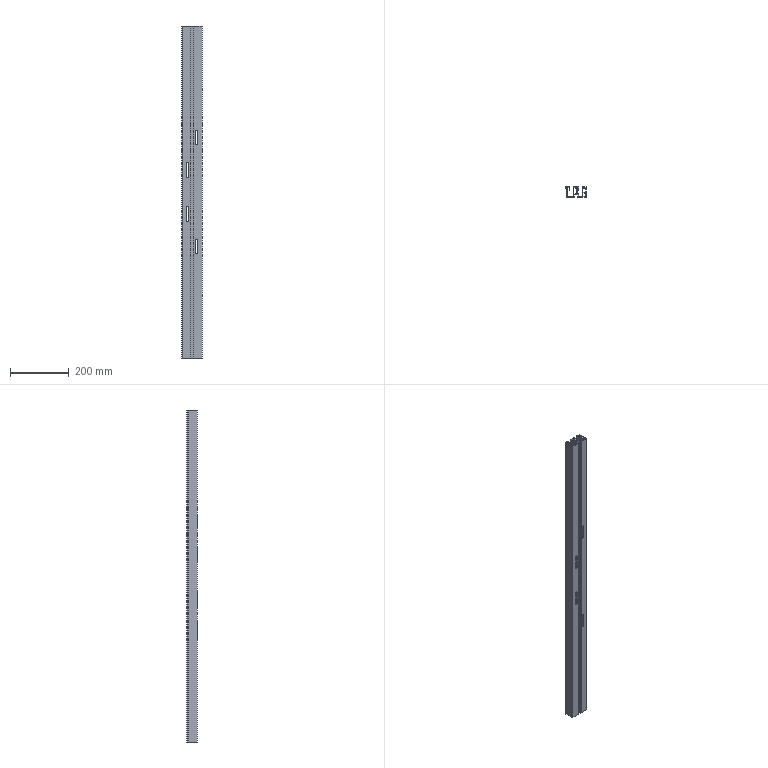Part | SolidWorks | features Cut 1, Extrusion 1, ICE 1 | 1 solid | 95 faces | box 70 x 35 x 1130 mm | volume 809219 mm3 | plane 66 | cylinder 29 | commonest cylinder face diameters 9 x12 2 x8 5 x4 3 x3 1 x1 4 x1